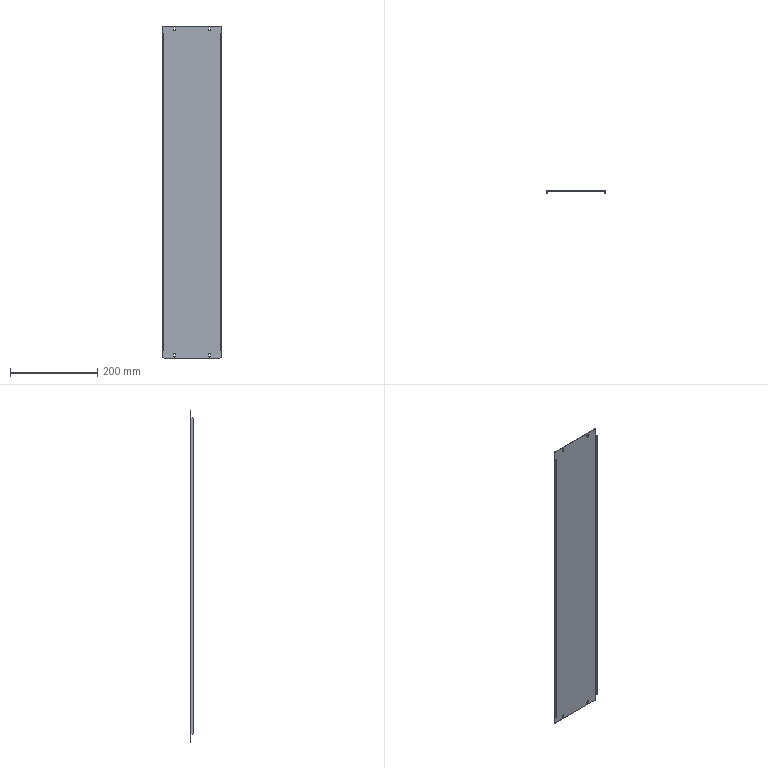Part | SolidWorks | features BaseBody 1 | 1 solid | 42 faces | box 134 x 7.2 x 760 mm | volume 132478 mm3 | plane 22 | cylinder 20 | commonest cylinder face diameters 4 x12 6 x8
STEP:
#1=CARTESIAN_POINT('',(40.,0.,-370.));
#2=VERTEX_POINT('',#1);
#3=CARTESIAN_POINT('',(40.,1.2,-370.));
#4=VERTEX_POINT('',#3);
#5=CARTESIAN_POINT('',(40.,-6.001,-370.));
#6=DIRECTION('',(0.,1.,0.));
#7=VECTOR('',#6,1000.);
#8=LINE('',#5,#7);
#9=EDGE_CURVE('',#2,#4,#8,.T.);
#10=ORIENTED_EDGE('',*,*,#9,.F.);
#11=CARTESIAN_POINT('',(38.,0.,-372.));
#12=VERTEX_POINT('',#11);
#13=CARTESIAN_POINT('',(40.,0.,-372.));
#14=DIRECTION('',(0.,-1.,0.));
#15=DIRECTION('',(0.,0.,1.));
#16=AXIS2_PLACEMENT_3D('',#13,#14,#15);
#17=CIRCLE('',#16,2.);
#18=EDGE_CURVE('',#2,#12,#17,.T.);
#19=ORIENTED_EDGE('',*,*,#18,.T.);
#20=CARTESIAN_POINT('',(38.,1.2,-372.));
#21=VERTEX_POINT('',#20);
#22=CARTESIAN_POINT('',(38.,-6.001,-372.));
#23=DIRECTION('',(0.,1.,0.));
#24=VECTOR('',#23,1000.);
#25=LINE('',#22,#24);
#26=EDGE_CURVE('',#12,#21,#25,.T.);
#27=ORIENTED_EDGE('',*,*,#26,.T.);
#28=CARTESIAN_POINT('',(40.,1.2,-372.));
#29=DIRECTION('',(0.,1.,0.));
#30=DIRECTION('',(0.,0.,1.));
#31=AXIS2_PLACEMENT_3D('',#28,#29,#30);
#32=CIRCLE('',#31,2.);
#33=EDGE_CURVE('',#21,#4,#32,.T.);
#34=ORIENTED_EDGE('',*,*,#33,.T.);
#35=EDGE_LOOP('',(#10,#19,#27,#34));
#36=FACE_OUTER_BOUND('',#35,.T.);
#37=CARTESIAN_POINT('',(40.,-6.001,-372.));
#38=DIRECTION('',(0.,1.,0.));
#39=DIRECTION('',(0.,0.,1.));
#40=AXIS2_PLACEMENT_3D('',#37,#38,#39);
#41=CYLINDRICAL_SURFACE('',#40,2.);
#42=ADVANCED_FACE('',(#36),#41,.F.);
#43=CARTESIAN_POINT('',(-40.,0.,-370.));
#44=VERTEX_POINT('',#43);
#45=CARTESIAN_POINT('',(-40.,1.2,-370.));
#46=VERTEX_POINT('',#45);
#47=CARTESIAN_POINT('',(-40.,-6.001,-370.));
#48=DIRECTION('',(0.,1.,0.));
#49=VECTOR('',#48,1000.);
#50=LINE('',#47,#49);
#51=EDGE_CURVE('',#44,#46,#50,.T.);
#52=ORIENTED_EDGE('',*,*,#51,.F.);
#53=CARTESIAN_POINT('',(-42.,0.,-372.));
#54=VERTEX_POINT('',#53);
#55=CARTESIAN_POINT('',(-40.,0.,-372.));
#56=DIRECTION('',(0.,-1.,0.));
#57=DIRECTION('',(0.,0.,1.));
#58=AXIS2_PLACEMENT_3D('',#55,#56,#57);
#59=CIRCLE('',#58,2.);
#60=EDGE_CURVE('',#44,#54,#59,.T.);
#61=ORIENTED_EDGE('',*,*,#60,.T.);
#62=CARTESIAN_POINT('',(-42.,1.2,-372.));
#63=VERTEX_POINT('',#62);
#64=CARTESIAN_POINT('',(-42.,-6.001,-372.));
#65=DIRECTION('',(0.,1.,0.));
#66=VECTOR('',#65,1000.);
#67=LINE('',#64,#66);
#68=EDGE_CURVE('',#54,#63,#67,.T.);
#69=ORIENTED_EDGE('',*,*,#68,.T.);
#70=CARTESIAN_POINT('',(-40.,1.2,-372.));
#71=DIRECTION('',(0.,1.,0.));
#72=DIRECTION('',(0.,0.,1.));
#73=AXIS2_PLACEMENT_3D('',#70,#71,#72);
#74=CIRCLE('',#73,2.);
#75=EDGE_CURVE('',#63,#46,#74,.T.);
#76=ORIENTED_EDGE('',*,*,#75,.T.);
#77=EDGE_LOOP('',(#52,#61,#69,#76));
#78=FACE_OUTER_BOUND('',#77,.T.);
#79=CARTESIAN_POINT('',(-40.,-6.001,-372.));
#80=DIRECTION('',(0.,1.,0.));
#81=DIRECTION('',(0.,0.,1.));
#82=AXIS2_PLACEMENT_3D('',#79,#80,#81);
#83=CYLINDRICAL_SURFACE('',#82,2.);
#84=ADVANCED_FACE('',(#78),#83,.F.);
#85=CARTESIAN_POINT('',(-42.,0.,372.));
#86=VERTEX_POINT('',#85);
#87=CARTESIAN_POINT('',(-38.,0.,372.));
#88=VERTEX_POINT('',#87);
#89=CARTESIAN_POINT('',(-40.,0.,372.));
#90=DIRECTION('',(0.,-1.,0.));
#91=DIRECTION('',(0.,0.,1.));
#92=AXIS2_PLACEMENT_3D('',#89,#90,#91);
#93=CIRCLE('',#92,2.);
#94=EDGE_CURVE('',#86,#88,#93,.T.);
#95=ORIENTED_EDGE('',*,*,#94,.T.);
#96=CARTESIAN_POINT('',(-38.,1.2,372.));
#97=VERTEX_POINT('',#96);
#98=CARTESIAN_POINT('',(-38.,-6.001,372.));
#99=DIRECTION('',(0.,1.,0.));
#100=VECTOR('',#99,1000.);
#101=LINE('',#98,#100);
#102=EDGE_CURVE('',#88,#97,#101,.T.);
#103=ORIENTED_EDGE('',*,*,#102,.T.);
#104=CARTESIAN_POINT('',(-42.,1.2,372.));
#105=VERTEX_POINT('',#104);
#106=CARTESIAN_POINT('',(-40.,1.2,372.));
#107=DIRECTION('',(0.,1.,0.));
#108=DIRECTION('',(0.,0.,1.));
#109=AXIS2_PLACEMENT_3D('',#106,#107,#108);
#110=CIRCLE('',#109,2.);
#111=EDGE_CURVE('',#97,#105,#110,.T.);
#112=ORIENTED_EDGE('',*,*,#111,.T.);
#113=CARTESIAN_POINT('',(-42.,-6.001,372.));
#114=DIRECTION('',(0.,1.,0.));
#115=VECTOR('',#114,1000.);
#116=LINE('',#113,#115);
#117=EDGE_CURVE('',#86,#105,#116,.T.);
#118=ORIENTED_EDGE('',*,*,#117,.F.);
#119=EDGE_LOOP('',(#95,#103,#112,#118));
#120=FACE_OUTER_BOUND('',#119,.T.);
#121=CARTESIAN_POINT('',(-40.,-6.001,372.));
#122=DIRECTION('',(0.,1.,0.));
#123=DIRECTION('',(0.,0.,1.));
#124=AXIS2_PLACEMENT_3D('',#121,#122,#123);
#125=CYLINDRICAL_SURFACE('',#124,2.);
#126=ADVANCED_FACE('',(#120),#125,.F.);
#127=CARTESIAN_POINT('',(40.,0.,378.));
#128=VERTEX_POINT('',#127);
#129=CARTESIAN_POINT('',(40.,1.2,378.));
#130=VERTEX_POINT('',#129);
#131=CARTESIAN_POINT('',(40.,-6.001,378.));
#132=DIRECTION('',(0.,1.,0.));
#133=VECTOR('',#132,1000.);
#134=LINE('',#131,#133);
#135=EDGE_CURVE('',#128,#130,#134,.T.);
#136=ORIENTED_EDGE('',*,*,#135,.F.);
#137=CARTESIAN_POINT('',(38.,0.,376.));
#138=VERTEX_POINT('',#137);
#139=CARTESIAN_POINT('',(40.,0.,376.));
#140=DIRECTION('',(0.,-1.,0.));
#141=DIRECTION('',(0.,0.,1.));
#142=AXIS2_PLACEMENT_3D('',#139,#140,#141);
#143=CIRCLE('',#142,2.);
#144=EDGE_CURVE('',#128,#138,#143,.T.);
#145=ORIENTED_EDGE('',*,*,#144,.T.);
#146=CARTESIAN_POINT('',(38.,1.2,376.));
#147=VERTEX_POINT('',#146);
#148=CARTESIAN_POINT('',(38.,-6.001,376.));
#149=DIRECTION('',(0.,1.,0.));
#150=VECTOR('',#149,1000.);
#151=LINE('',#148,#150);
#152=EDGE_CURVE('',#138,#147,#151,.T.);
#153=ORIENTED_EDGE('',*,*,#152,.T.);
#154=CARTESIAN_POINT('',(40.,1.2,376.));
#155=DIRECTION('',(0.,1.,0.));
#156=DIRECTION('',(0.,0.,1.));
#157=AXIS2_PLACEMENT_3D('',#154,#155,#156);
#158=CIRCLE('',#157,2.);
#159=EDGE_CURVE('',#147,#130,#158,.T.);
#160=ORIENTED_EDGE('',*,*,#159,.T.);
#161=EDGE_LOOP('',(#136,#145,#153,#160));
#162=FACE_OUTER_BOUND('',#161,.T.);
#163=CARTESIAN_POINT('',(40.,-6.001,376.));
#164=DIRECTION('',(0.,1.,0.));
#165=DIRECTION('',(0.,0.,1.));
#166=AXIS2_PLACEMENT_3D('',#163,#164,#165);
#167=CYLINDRICAL_SURFACE('',#166,2.);
#168=ADVANCED_FACE('',(#162),#167,.F.);
#169=CARTESIAN_POINT('',(38.,0.,372.));
#170=VERTEX_POINT('',#169);
#171=CARTESIAN_POINT('',(38.,0.,372.));
#172=DIRECTION('',(0.,0.,-1.));
#173=VECTOR('',#172,1000.);
#174=LINE('',#171,#173);
#175=EDGE_CURVE('',#138,#170,#174,.T.);
#176=ORIENTED_EDGE('',*,*,#175,.T.);
#177=CARTESIAN_POINT('',(38.,1.2,372.));
#178=VERTEX_POINT('',#177);
#179=CARTESIAN_POINT('',(38.,-6.001,372.));
#180=DIRECTION('',(0.,1.,0.));
#181=VECTOR('',#180,1000.);
#182=LINE('',#179,#181);
#183=EDGE_CURVE('',#170,#178,#182,.T.);
#184=ORIENTED_EDGE('',*,*,#183,.T.);
#185=CARTESIAN_POINT('',(38.,1.2,372.));
#186=DIRECTION('',(0.,0.,1.));
#187=VECTOR('',#186,1000.);
#188=LINE('',#185,#187);
#189=EDGE_CURVE('',#178,#147,#188,.T.);
#190=ORIENTED_EDGE('',*,*,#189,.T.);
#191=ORIENTED_EDGE('',*,*,#152,.F.);
#192=EDGE_LOOP('',(#176,#184,#190,#191));
#193=FACE_OUTER_BOUND('',#192,.T.);
#194=CARTESIAN_POINT('',(38.,-6.001,372.));
#195=DIRECTION('',(-1.,0.,0.));
#196=DIRECTION('',(0.,0.,1.));
#197=AXIS2_PLACEMENT_3D('',#194,#195,#196);
#198=PLANE('',#197);
#199=ADVANCED_FACE('',(#193),#198,.F.);
#200=CARTESIAN_POINT('',(42.,0.,372.));
#201=VERTEX_POINT('',#200);
#202=CARTESIAN_POINT('',(42.,0.,376.));
#203=VERTEX_POINT('',#202);
#204=CARTESIAN_POINT('',(42.,0.,372.));
#205=DIRECTION('',(0.,0.,1.));
#206=VECTOR('',#205,1000.);
#207=LINE('',#204,#206);
#208=EDGE_CURVE('',#201,#203,#207,.T.);
#209=ORIENTED_EDGE('',*,*,#208,.T.);
#210=CARTESIAN_POINT('',(42.,1.2,376.));
#211=VERTEX_POINT('',#210);
#212=CARTESIAN_POINT('',(42.,-6.001,376.));
#213=DIRECTION('',(0.,1.,0.));
#214=VECTOR('',#213,1000.);
#215=LINE('',#212,#214);
#216=EDGE_CURVE('',#203,#211,#215,.T.);
#217=ORIENTED_EDGE('',*,*,#216,.T.);
#218=CARTESIAN_POINT('',(42.,1.2,372.));
#219=VERTEX_POINT('',#218);
#220=CARTESIAN_POINT('',(42.,1.2,372.));
#221=DIRECTION('',(0.,0.,-1.));
#222=VECTOR('',#221,1000.);
#223=LINE('',#220,#222);
#224=EDGE_CURVE('',#211,#219,#223,.T.);
#225=ORIENTED_EDGE('',*,*,#224,.T.);
#226=CARTESIAN_POINT('',(42.,-6.001,372.));
#227=DIRECTION('',(0.,1.,0.));
#228=VECTOR('',#227,1000.);
#229=LINE('',#226,#228);
#230=EDGE_CURVE('',#201,#219,#229,.T.);
#231=ORIENTED_EDGE('',*,*,#230,.F.);
#232=EDGE_LOOP('',(#209,#217,#225,#231));
#233=FACE_OUTER_BOUND('',#232,.T.);
#234=CARTESIAN_POINT('',(42.,-6.001,372.));
#235=DIRECTION('',(1.,0.,0.));
#236=DIRECTION('',(0.,1.,0.));
#237=AXIS2_PLACEMENT_3D('',#234,#235,#236);
#238=PLANE('',#237);
#239=ADVANCED_FACE('',(#233),#238,.F.);
#240=CARTESIAN_POINT('',(40.,0.,372.));
#241=DIRECTION('',(0.,-1.,0.));
#242=DIRECTION('',(0.,0.,1.));
#243=AXIS2_PLACEMENT_3D('',#240,#241,#242);
#244=CIRCLE('',#243,2.);
#245=EDGE_CURVE('',#170,#201,#244,.T.);
#246=ORIENTED_EDGE('',*,*,#245,.T.);
#247=ORIENTED_EDGE('',*,*,#230,.T.);
#248=CARTESIAN_POINT('',(40.,1.2,372.));
#249=DIRECTION('',(0.,1.,0.));
#250=DIRECTION('',(0.,0.,1.));
#251=AXIS2_PLACEMENT_3D('',#248,#249,#250);
#252=CIRCLE('',#251,2.);
#253=EDGE_CURVE('',#219,#178,#252,.T.);
#254=ORIENTED_EDGE('',*,*,#253,.T.);
#255=ORIENTED_EDGE('',*,*,#183,.F.);
#256=EDGE_LOOP('',(#246,#247,#254,#255));
#257=FACE_OUTER_BOUND('',#256,.T.);
#258=CARTESIAN_POINT('',(40.,-6.001,372.));
#259=DIRECTION('',(0.,1.,0.));
#260=DIRECTION('',(0.,0.,1.));
#261=AXIS2_PLACEMENT_3D('',#258,#259,#260);
#262=CYLINDRICAL_SURFACE('',#261,2.);
#263=ADVANCED_FACE('',(#257),#262,.F.);
#264=CARTESIAN_POINT('',(-38.,0.,376.));
#265=VERTEX_POINT('',#264);
#266=CARTESIAN_POINT('',(-38.,0.,372.));
#267=DIRECTION('',(0.,0.,1.));
#268=VECTOR('',#267,1000.);
#269=LINE('',#266,#268);
#270=EDGE_CURVE('',#88,#265,#269,.T.);
#271=ORIENTED_EDGE('',*,*,#270,.T.);
#272=CARTESIAN_POINT('',(-38.,1.2,376.));
#273=VERTEX_POINT('',#272);
#274=CARTESIAN_POINT('',(-38.,-6.001,376.));
#275=DIRECTION('',(0.,1.,0.));
#276=VECTOR('',#275,1000.);
#277=LINE('',#274,#276);
#278=EDGE_CURVE('',#265,#273,#277,.T.);
#279=ORIENTED_EDGE('',*,*,#278,.T.);
#280=CARTESIAN_POINT('',(-38.,1.2,372.));
#281=DIRECTION('',(0.,0.,-1.));
#282=VECTOR('',#281,1000.);
#283=LINE('',#280,#282);
#284=EDGE_CURVE('',#273,#97,#283,.T.);
#285=ORIENTED_EDGE('',*,*,#284,.T.);
#286=ORIENTED_EDGE('',*,*,#102,.F.);
#287=EDGE_LOOP('',(#271,#279,#285,#286));
#288=FACE_OUTER_BOUND('',#287,.T.);
#289=CARTESIAN_POINT('',(-38.,-6.001,372.));
#290=DIRECTION('',(1.,0.,0.));
#291=DIRECTION('',(0.,1.,0.));
#292=AXIS2_PLACEMENT_3D('',#289,#290,#291);
#293=PLANE('',#292);
#294=ADVANCED_FACE('',(#288),#293,.F.);
#295=CARTESIAN_POINT('',(-40.,0.,378.));
#296=VERTEX_POINT('',#295);
#297=CARTESIAN_POINT('',(-40.,1.2,378.));
#298=VERTEX_POINT('',#297);
#299=CARTESIAN_POINT('',(-40.,-6.001,378.));
#300=DIRECTION('',(0.,1.,0.));
#301=VECTOR('',#300,1000.);
#302=LINE('',#299,#301);
#303=EDGE_CURVE('',#296,#298,#302,.T.);
#304=ORIENTED_EDGE('',*,*,#303,.F.);
#305=CARTESIAN_POINT('',(-42.,0.,376.));
#306=VERTEX_POINT('',#305);
#307=CARTESIAN_POINT('',(-40.,0.,376.));
#308=DIRECTION('',(0.,-1.,0.));
#309=DIRECTION('',(0.,0.,1.));
#310=AXIS2_PLACEMENT_3D('',#307,#308,#309);
#311=CIRCLE('',#310,2.);
#312=EDGE_CURVE('',#296,#306,#311,.T.);
#313=ORIENTED_EDGE('',*,*,#312,.T.);
#314=CARTESIAN_POINT('',(-42.,1.2,376.));
#315=VERTEX_POINT('',#314);
#316=CARTESIAN_POINT('',(-42.,-6.001,376.));
#317=DIRECTION('',(0.,1.,0.));
#318=VECTOR('',#317,1000.);
#319=LINE('',#316,#318);
#320=EDGE_CURVE('',#306,#315,#319,.T.);
#321=ORIENTED_EDGE('',*,*,#320,.T.);
#322=CARTESIAN_POINT('',(-40.,1.2,376.));
#323=DIRECTION('',(0.,1.,0.));
#324=DIRECTION('',(0.,0.,1.));
#325=AXIS2_PLACEMENT_3D('',#322,#323,#324);
#326=CIRCLE('',#325,2.);
#327=EDGE_CURVE('',#315,#298,#326,.T.);
#328=ORIENTED_EDGE('',*,*,#327,.T.);
#329=EDGE_LOOP('',(#304,#313,#321,#328));
#330=FACE_OUTER_BOUND('',#329,.T.);
#331=CARTESIAN_POINT('',(-40.,-6.001,376.));
#332=DIRECTION('',(0.,1.,0.));
#333=DIRECTION('',(0.,0.,1.));
#334=AXIS2_PLACEMENT_3D('',#331,#332,#333);
#335=CYLINDRICAL_SURFACE('',#334,2.);
#336=ADVANCED_FACE('',(#330),#335,.F.);
#337=CARTESIAN_POINT('',(-42.,0.,372.));
#338=DIRECTION('',(0.,0.,-1.));
#339=VECTOR('',#338,1000.);
#340=LINE('',#337,#339);
#341=EDGE_CURVE('',#306,#86,#340,.T.);
#342=ORIENTED_EDGE('',*,*,#341,.T.);
#343=ORIENTED_EDGE('',*,*,#117,.T.);
#344=CARTESIAN_POINT('',(-42.,1.2,372.));
#345=DIRECTION('',(0.,0.,1.));
#346=VECTOR('',#345,1000.);
#347=LINE('',#344,#346);
#348=EDGE_CURVE('',#105,#315,#347,.T.);
#349=ORIENTED_EDGE('',*,*,#348,.T.);
#350=ORIENTED_EDGE('',*,*,#320,.F.);
#351=EDGE_LOOP('',(#342,#343,#349,#350));
#352=FACE_OUTER_BOUND('',#351,.T.);
#353=CARTESIAN_POINT('',(-42.,-6.001,372.));
#354=DIRECTION('',(-1.,0.,0.));
#355=DIRECTION('',(0.,0.,1.));
#356=AXIS2_PLACEMENT_3D('',#353,#354,#355);
#357=PLANE('',#356);
#358=ADVANCED_FACE('',(#352),#357,.F.);
#359=CARTESIAN_POINT('',(-42.,0.,-376.));
#360=VERTEX_POINT('',#359);
#361=CARTESIAN_POINT('',(-42.,0.,-376.));
#362=DIRECTION('',(0.,0.,-1.));
#363=VECTOR('',#362,1000.);
#364=LINE('',#361,#363);
#365=EDGE_CURVE('',#54,#360,#364,.T.);
#366=ORIENTED_EDGE('',*,*,#365,.T.);
#367=CARTESIAN_POINT('',(-42.,1.2,-376.));
#368=VERTEX_POINT('',#367);
#369=CARTESIAN_POINT('',(-42.,-6.001,-376.));
#370=DIRECTION('',(0.,1.,0.));
#371=VECTOR('',#370,1000.);
#372=LINE('',#369,#371);
#373=EDGE_CURVE('',#360,#368,#372,.T.);
#374=ORIENTED_EDGE('',*,*,#373,.T.);
#375=CARTESIAN_POINT('',(-42.,1.2,-376.));
#376=DIRECTION('',(0.,0.,1.));
#377=VECTOR('',#376,1000.);
#378=LINE('',#375,#377);
#379=EDGE_CURVE('',#368,#63,#378,.T.);
#380=ORIENTED_EDGE('',*,*,#379,.T.);
#381=ORIENTED_EDGE('',*,*,#68,.F.);
#382=EDGE_LOOP('',(#366,#374,#380,#381));
#383=FACE_OUTER_BOUND('',#382,.T.);
#384=CARTESIAN_POINT('',(-42.,-6.001,-376.));
#385=DIRECTION('',(-1.,0.,0.));
#386=DIRECTION('',(0.,0.,1.));
#387=AXIS2_PLACEMENT_3D('',#384,#385,#386);
#388=PLANE('',#387);
#389=ADVANCED_FACE('',(#383),#388,.F.);
#390=CARTESIAN_POINT('',(-38.,0.,-376.));
#391=VERTEX_POINT('',#390);
#392=CARTESIAN_POINT('',(-38.,0.,-372.));
#393=VERTEX_POINT('',#392);
#394=CARTESIAN_POINT('',(-38.,0.,-376.));
#395=DIRECTION('',(0.,0.,1.));
#396=VECTOR('',#395,1000.);
#397=LINE('',#394,#396);
#398=EDGE_CURVE('',#391,#393,#397,.T.);
#399=ORIENTED_EDGE('',*,*,#398,.T.);
#400=CARTESIAN_POINT('',(-38.,1.2,-372.));
#401=VERTEX_POINT('',#400);
#402=CARTESIAN_POINT('',(-38.,-6.001,-372.));
#403=DIRECTION('',(0.,1.,0.));
#404=VECTOR('',#403,1000.);
#405=LINE('',#402,#404);
#406=EDGE_CURVE('',#393,#401,#405,.T.);
#407=ORIENTED_EDGE('',*,*,#406,.T.);
#408=CARTESIAN_POINT('',(-38.,1.2,-376.));
#409=VERTEX_POINT('',#408);
#410=CARTESIAN_POINT('',(-38.,1.2,-376.));
#411=DIRECTION('',(0.,0.,-1.));
#412=VECTOR('',#411,1000.);
#413=LINE('',#410,#412);
#414=EDGE_CURVE('',#401,#409,#413,.T.);
#415=ORIENTED_EDGE('',*,*,#414,.T.);
#416=CARTESIAN_POINT('',(-38.,-6.001,-376.));
#417=DIRECTION('',(0.,1.,0.));
#418=VECTOR('',#417,1000.);
#419=LINE('',#416,#418);
#420=EDGE_CURVE('',#391,#409,#419,.T.);
#421=ORIENTED_EDGE('',*,*,#420,.F.);
#422=EDGE_LOOP('',(#399,#407,#415,#421));
#423=FACE_OUTER_BOUND('',#422,.T.);
#424=CARTESIAN_POINT('',(-38.,-6.001,-376.));
#425=DIRECTION('',(1.,0.,0.));
#426=DIRECTION('',(0.,1.,0.));
#427=AXIS2_PLACEMENT_3D('',#424,#425,#426);
#428=PLANE('',#427);
#429=ADVANCED_FACE('',(#423),#428,.F.);
#430=CARTESIAN_POINT('',(-40.,0.,-376.));
#431=DIRECTION('',(0.,-1.,0.));
#432=DIRECTION('',(0.,0.,1.));
#433=AXIS2_PLACEMENT_3D('',#430,#431,#432);
#434=CIRCLE('',#433,2.);
#435=EDGE_CURVE('',#360,#391,#434,.T.);
#436=ORIENTED_EDGE('',*,*,#435,.T.);
#437=ORIENTED_EDGE('',*,*,#420,.T.);
#438=CARTESIAN_POINT('',(-40.,1.2,-376.));
#439=DIRECTION('',(0.,1.,0.));
#440=DIRECTION('',(0.,0.,1.));
#441=AXIS2_PLACEMENT_3D('',#438,#439,#440);
#442=CIRCLE('',#441,2.);
#443=EDGE_CURVE('',#409,#368,#442,.T.);
#444=ORIENTED_EDGE('',*,*,#443,.T.);
#445=ORIENTED_EDGE('',*,*,#373,.F.);
#446=EDGE_LOOP('',(#436,#437,#444,#445));
#447=FACE_OUTER_BOUND('',#446,.T.);
#448=CARTESIAN_POINT('',(-40.,-6.001,-376.));
#449=DIRECTION('',(0.,1.,0.));
#450=DIRECTION('',(0.,0.,1.));
#451=AXIS2_PLACEMENT_3D('',#448,#449,#450);
#452=CYLINDRICAL_SURFACE('',#451,2.);
#453=ADVANCED_FACE('',(#447),#452,.F.);
#454=CARTESIAN_POINT('',(38.,0.,-376.));
#455=VERTEX_POINT('',#454);
#456=CARTESIAN_POINT('',(38.,0.,-376.));
#457=DIRECTION('',(0.,0.,-1.));
#458=VECTOR('',#457,1000.);
#459=LINE('',#456,#458);
#460=EDGE_CURVE('',#12,#455,#459,.T.);
#461=ORIENTED_EDGE('',*,*,#460,.T.);
#462=CARTESIAN_POINT('',(38.,1.2,-376.));
#463=VERTEX_POINT('',#462);
#464=CARTESIAN_POINT('',(38.,-6.001,-376.));
#465=DIRECTION('',(0.,1.,0.));
#466=VECTOR('',#465,1000.);
#467=LINE('',#464,#466);
#468=EDGE_CURVE('',#455,#463,#467,.T.);
#469=ORIENTED_EDGE('',*,*,#468,.T.);
#470=CARTESIAN_POINT('',(38.,1.2,-376.));
#471=DIRECTION('',(0.,0.,1.));
#472=VECTOR('',#471,1000.);
#473=LINE('',#470,#472);
#474=EDGE_CURVE('',#463,#21,#473,.T.);
#475=ORIENTED_EDGE('',*,*,#474,.T.);
#476=ORIENTED_EDGE('',*,*,#26,.F.);
#477=EDGE_LOOP('',(#461,#469,#475,#476));
#478=FACE_OUTER_BOUND('',#477,.T.);
#479=CARTESIAN_POINT('',(38.,-6.001,-376.));
#480=DIRECTION('',(-1.,0.,0.));
#481=DIRECTION('',(0.,0.,1.));
#482=AXIS2_PLACEMENT_3D('',#479,#480,#481);
#483=PLANE('',#482);
#484=ADVANCED_FACE('',(#478),#483,.F.);
#485=CARTESIAN_POINT('',(42.,0.,-376.));
#486=VERTEX_POINT('',#485);
#487=CARTESIAN_POINT('',(42.,0.,-372.));
#488=VERTEX_POINT('',#487);
#489=CARTESIAN_POINT('',(42.,0.,-376.));
#490=DIRECTION('',(0.,0.,1.));
#491=VECTOR('',#490,1000.);
#492=LINE('',#489,#491);
#493=EDGE_CURVE('',#486,#488,#492,.T.);
#494=ORIENTED_EDGE('',*,*,#493,.T.);
#495=CARTESIAN_POINT('',(42.,1.2,-372.));
#496=VERTEX_POINT('',#495);
#497=CARTESIAN_POINT('',(42.,-6.001,-372.));
#498=DIRECTION('',(0.,1.,0.));
#499=VECTOR('',#498,1000.);
#500=LINE('',#497,#499);
#501=EDGE_CURVE('',#488,#496,#500,.T.);
#502=ORIENTED_EDGE('',*,*,#501,.T.);
#503=CARTESIAN_POINT('',(42.,1.2,-376.));
#504=VERTEX_POINT('',#503);
#505=CARTESIAN_POINT('',(42.,1.2,-376.));
#506=DIRECTION('',(0.,0.,-1.));
#507=VECTOR('',#506,1000.);
#508=LINE('',#505,#507);
#509=EDGE_CURVE('',#496,#504,#508,.T.);
#510=ORIENTED_EDGE('',*,*,#509,.T.);
#511=CARTESIAN_POINT('',(42.,-6.001,-376.));
#512=DIRECTION('',(0.,1.,0.));
#513=VECTOR('',#512,1000.);
#514=LINE('',#511,#513);
#515=EDGE_CURVE('',#486,#504,#514,.T.);
#516=ORIENTED_EDGE('',*,*,#515,.F.);
#517=EDGE_LOOP('',(#494,#502,#510,#516));
#518=FACE_OUTER_BOUND('',#517,.T.);
#519=CARTESIAN_POINT('',(42.,-6.001,-376.));
#520=DIRECTION('',(1.,0.,0.));
#521=DIRECTION('',(0.,1.,0.));
#522=AXIS2_PLACEMENT_3D('',#519,#520,#521);
#523=PLANE('',#522);
#524=ADVANCED_FACE('',(#518),#523,.F.);
#525=CARTESIAN_POINT('',(40.,0.,-376.));
#526=DIRECTION('',(0.,-1.,0.));
#527=DIRECTION('',(0.,0.,1.));
#528=AXIS2_PLACEMENT_3D('',#525,#526,#527);
#529=CIRCLE('',#528,2.);
#530=EDGE_CURVE('',#455,#486,#529,.T.);
#531=ORIENTED_EDGE('',*,*,#530,.T.);
#532=ORIENTED_EDGE('',*,*,#515,.T.);
#533=CARTESIAN_POINT('',(40.,1.2,-376.));
#534=DIRECTION('',(0.,1.,0.));
#535=DIRECTION('',(0.,0.,1.));
#536=AXIS2_PLACEMENT_3D('',#533,#534,#535);
#537=CIRCLE('',#536,2.);
#538=EDGE_CURVE('',#504,#463,#537,.T.);
#539=ORIENTED_EDGE('',*,*,#538,.T.);
#540=ORIENTED_EDGE('',*,*,#468,.F.);
#541=EDGE_LOOP('',(#531,#532,#539,#540));
#542=FACE_OUTER_BOUND('',#541,.T.);
#543=CARTESIAN_POINT('',(40.,-6.001,-376.));
#544=DIRECTION('',(0.,1.,0.));
#545=DIRECTION('',(0.,0.,1.));
#546=AXIS2_PLACEMENT_3D('',#543,#544,#545);
#547=CYLINDRICAL_SURFACE('',#546,2.);
#548=ADVANCED_FACE('',(#542),#547,.F.);
#549=CARTESIAN_POINT('',(64.,1.2,380.));
#550=VERTEX_POINT('',#549);
#551=CARTESIAN_POINT('',(67.,1.2,377.));
#552=VERTEX_POINT('',#551);
#553=CARTESIAN_POINT('',(64.,1.2,377.));
#554=DIRECTION('',(0.,1.,0.));
#555=DIRECTION('',(0.,0.,1.));
#556=AXIS2_PLACEMENT_3D('',#553,#554,#555);
#557=CIRCLE('',#556,3.);
#558=EDGE_CURVE('',#550,#552,#557,.T.);
#559=ORIENTED_EDGE('',*,*,#558,.F.);
#560=CARTESIAN_POINT('',(64.,0.,380.));
#561=VERTEX_POINT('',#560);
#562=CARTESIAN_POINT('',(64.,1.2,380.));
#563=DIRECTION('',(0.,1.,0.));
#564=VECTOR('',#563,1000.);
#565=LINE('',#562,#564);
#566=EDGE_CURVE('',#561,#550,#565,.T.);
#567=ORIENTED_EDGE('',*,*,#566,.F.);
#568=CARTESIAN_POINT('',(67.,0.,377.));
#569=VERTEX_POINT('',#568);
#570=CARTESIAN_POINT('',(64.,0.,377.));
#571=DIRECTION('',(0.,-1.,0.));
#572=DIRECTION('',(0.,0.,1.));
#573=AXIS2_PLACEMENT_3D('',#570,#571,#572);
#574=CIRCLE('',#573,3.);
#575=EDGE_CURVE('',#569,#561,#574,.T.);
#576=ORIENTED_EDGE('',*,*,#575,.F.);
#577=CARTESIAN_POINT('',(67.,1.2,377.));
#578=DIRECTION('',(0.,-1.,0.));
#579=VECTOR('',#578,1000.);
#580=LINE('',#577,#579);
#581=EDGE_CURVE('',#552,#569,#580,.T.);
#582=ORIENTED_EDGE('',*,*,#581,.F.);
#583=EDGE_LOOP('',(#559,#567,#576,#582));
#584=FACE_OUTER_BOUND('',#583,.T.);
#585=CARTESIAN_POINT('',(64.,1.2,377.));
#586=DIRECTION('',(0.,-1.,0.));
#587=DIRECTION('',(0.,0.,-1.));
#588=AXIS2_PLACEMENT_3D('',#585,#586,#587);
#589=CYLINDRICAL_SURFACE('',#588,3.);
#590=ADVANCED_FACE('',(#584),#589,.T.);
#591=CARTESIAN_POINT('',(65.8,-6.,359.));
#592=VERTEX_POINT('',#591);
#593=CARTESIAN_POINT('',(65.8,-3.,362.));
#594=VERTEX_POINT('',#593);
#595=CARTESIAN_POINT('',(65.8,-3.,359.));
#596=DIRECTION('',(-1.,0.,0.));
#597=DIRECTION('',(0.,0.,-1.));
#598=AXIS2_PLACEMENT_3D('',#595,#596,#597);
#599=CIRCLE('',#598,3.);
#600=EDGE_CURVE('',#592,#594,#599,.T.);
#601=ORIENTED_EDGE('',*,*,#600,.F.);
#602=CARTESIAN_POINT('',(67.,-6.,359.));
#603=VERTEX_POINT('',#602);
#604=CARTESIAN_POINT('',(0.,-6.,359.));
#605=DIRECTION('',(-1.,0.,0.));
#606=VECTOR('',#605,1000.);
#607=LINE('',#604,#606);
#608=EDGE_CURVE('',#603,#592,#607,.T.);
#609=ORIENTED_EDGE('',*,*,#608,.F.);
#610=CARTESIAN_POINT('',(67.,-3.,362.));
#611=VERTEX_POINT('',#610);
#612=CARTESIAN_POINT('',(67.,-3.,359.));
#613=DIRECTION('',(1.,0.,0.));
#614=DIRECTION('',(0.,0.,1.));
#615=AXIS2_PLACEMENT_3D('',#612,#613,#614);
#616=CIRCLE('',#615,3.);
#617=EDGE_CURVE('',#611,#603,#616,.T.);
#618=ORIENTED_EDGE('',*,*,#617,.F.);
#619=CARTESIAN_POINT('',(-67.,-3.,362.));
#620=DIRECTION('',(1.,0.,0.));
#621=VECTOR('',#620,1000.);
#622=LINE('',#619,#621);
#623=EDGE_CURVE('',#594,#611,#622,.T.);
#624=ORIENTED_EDGE('',*,*,#623,.F.);
#625=EDGE_LOOP('',(#601,#609,#618,#624));
#626=FACE_OUTER_BOUND('',#625,.T.);
#627=CARTESIAN_POINT('',(-67.,-3.,359.));
#628=DIRECTION('',(1.,0.,0.));
#629=DIRECTION('',(0.,0.,-1.));
#630=AXIS2_PLACEMENT_3D('',#627,#628,#629);
#631=CYLINDRICAL_SURFACE('',#630,3.);
#632=ADVANCED_FACE('',(#626),#631,.T.);
#633=CARTESIAN_POINT('',(-67.,1.2,377.));
#634=VERTEX_POINT('',#633);
#635=CARTESIAN_POINT('',(-64.,1.2,380.));
#636=VERTEX_POINT('',#635);
#637=CARTESIAN_POINT('',(-64.,1.2,377.));
#638=DIRECTION('',(0.,1.,0.));
#639=DIRECTION('',(0.,0.,1.));
#640=AXIS2_PLACEMENT_3D('',#637,#638,#639);
#641=CIRCLE('',#640,3.);
#642=EDGE_CURVE('',#634,#636,#641,.T.);
#643=ORIENTED_EDGE('',*,*,#642,.F.);
#644=CARTESIAN_POINT('',(-67.,0.,377.));
#645=VERTEX_POINT('',#644);
#646=CARTESIAN_POINT('',(-67.,1.2,377.));
#647=DIRECTION('',(0.,1.,0.));
#648=VECTOR('',#647,1000.);
#649=LINE('',#646,#648);
#650=EDGE_CURVE('',#645,#634,#649,.T.);
#651=ORIENTED_EDGE('',*,*,#650,.F.);
#652=CARTESIAN_POINT('',(-64.,0.,380.));
#653=VERTEX_POINT('',#652);
#654=CARTESIAN_POINT('',(-64.,0.,377.));
#655=DIRECTION('',(0.,-1.,0.));
#656=DIRECTION('',(0.,0.,1.));
#657=AXIS2_PLACEMENT_3D('',#654,#655,#656);
#658=CIRCLE('',#657,3.);
#659=EDGE_CURVE('',#653,#645,#658,.T.);
#660=ORIENTED_EDGE('',*,*,#659,.F.);
#661=CARTESIAN_POINT('',(-64.,1.2,380.));
#662=DIRECTION('',(0.,-1.,0.));
#663=VECTOR('',#662,1000.);
#664=LINE('',#661,#663);
#665=EDGE_CURVE('',#636,#653,#664,.T.);
#666=ORIENTED_EDGE('',*,*,#665,.F.);
#667=EDGE_LOOP('',(#643,#651,#660,#666));
#668=FACE_OUTER_BOUND('',#667,.T.);
#669=CARTESIAN_POINT('',(-64.,1.2,377.));
#670=DIRECTION('',(0.,-1.,0.));
#671=DIRECTION('',(0.,0.,-1.));
#672=AXIS2_PLACEMENT_3D('',#669,#670,#671);
#673=CYLINDRICAL_SURFACE('',#672,3.);
#674=ADVANCED_FACE('',(#668),#673,.T.);
#675=CARTESIAN_POINT('',(-67.,-6.,359.));
#676=VERTEX_POINT('',#675);
#677=CARTESIAN_POINT('',(-67.,-3.,362.));
#678=VERTEX_POINT('',#677);
#679=CARTESIAN_POINT('',(-67.,-3.,359.));
#680=DIRECTION('',(-1.,0.,0.));
#681=DIRECTION('',(0.,0.,-1.));
#682=AXIS2_PLACEMENT_3D('',#679,#680,#681);
#683=CIRCLE('',#682,3.);
#684=EDGE_CURVE('',#676,#678,#683,.T.);
#685=ORIENTED_EDGE('',*,*,#684,.F.);
#686=CARTESIAN_POINT('',(-65.8,-6.,359.));
#687=VERTEX_POINT('',#686);
#688=CARTESIAN_POINT('',(0.,-6.,359.));
#689=DIRECTION('',(-1.,0.,0.));
#690=VECTOR('',#689,1000.);
#691=LINE('',#688,#690);
#692=EDGE_CURVE('',#687,#676,#691,.T.);
#693=ORIENTED_EDGE('',*,*,#692,.F.);
#694=CARTESIAN_POINT('',(-65.8,-3.,362.));
#695=VERTEX_POINT('',#694);
#696=CARTESIAN_POINT('',(-65.8,-3.,359.));
#697=DIRECTION('',(1.,0.,0.));
#698=DIRECTION('',(0.,0.,-1.));
#699=AXIS2_PLACEMENT_3D('',#696,#697,#698);
#700=CIRCLE('',#699,3.);
#701=EDGE_CURVE('',#695,#687,#700,.T.);
#702=ORIENTED_EDGE('',*,*,#701,.F.);
#703=CARTESIAN_POINT('',(-67.,-3.,362.));
#704=DIRECTION('',(1.,0.,0.));
#705=VECTOR('',#704,1000.);
#706=LINE('',#703,#705);
#707=EDGE_CURVE('',#678,#695,#706,.T.);
#708=ORIENTED_EDGE('',*,*,#707,.F.);
#709=EDGE_LOOP('',(#685,#693,#702,#708));
#710=FACE_OUTER_BOUND('',#709,.T.);
#711=CARTESIAN_POINT('',(-67.,-3.,359.));
#712=DIRECTION('',(1.,0.,0.));
#713=DIRECTION('',(0.,0.,-1.));
#714=AXIS2_PLACEMENT_3D('',#711,#712,#713);
#715=CYLINDRICAL_SURFACE('',#714,3.);
#716=ADVANCED_FACE('',(#710),#715,.T.);
#717=CARTESIAN_POINT('',(-64.,1.2,-380.));
#718=VERTEX_POINT('',#717);
#719=CARTESIAN_POINT('',(-67.,1.2,-377.));
#720=VERTEX_POINT('',#719);
#721=CARTESIAN_POINT('',(-64.,1.2,-377.));
#722=DIRECTION('',(0.,1.,0.));
#723=DIRECTION('',(0.,0.,1.));
#724=AXIS2_PLACEMENT_3D('',#721,#722,#723);
#725=CIRCLE('',#724,3.);
#726=EDGE_CURVE('',#718,#720,#725,.T.);
#727=ORIENTED_EDGE('',*,*,#726,.F.);
#728=CARTESIAN_POINT('',(-64.,0.,-380.));
#729=VERTEX_POINT('',#728);
#730=CARTESIAN_POINT('',(-64.,1.2,-380.));
#731=DIRECTION('',(0.,1.,0.));
#732=VECTOR('',#731,1000.);
#733=LINE('',#730,#732);
#734=EDGE_CURVE('',#729,#718,#733,.T.);
#735=ORIENTED_EDGE('',*,*,#734,.F.);
#736=CARTESIAN_POINT('',(-67.,0.,-377.));
#737=VERTEX_POINT('',#736);
#738=CARTESIAN_POINT('',(-64.,0.,-377.));
#739=DIRECTION('',(0.,-1.,0.));
#740=DIRECTION('',(0.,0.,1.));
#741=AXIS2_PLACEMENT_3D('',#738,#739,#740);
#742=CIRCLE('',#741,3.);
#743=EDGE_CURVE('',#737,#729,#742,.T.);
#744=ORIENTED_EDGE('',*,*,#743,.F.);
#745=CARTESIAN_POINT('',(-67.,1.2,-377.));
#746=DIRECTION('',(0.,-1.,0.));
#747=VECTOR('',#746,1000.);
#748=LINE('',#745,#747);
#749=EDGE_CURVE('',#720,#737,#748,.T.);
#750=ORIENTED_EDGE('',*,*,#749,.F.);
#751=EDGE_LOOP('',(#727,#735,#744,#750));
#752=FACE_OUTER_BOUND('',#751,.T.);
#753=CARTESIAN_POINT('',(-64.,1.2,-377.));
#754=DIRECTION('',(0.,-1.,0.));
#755=DIRECTION('',(0.,0.,-1.));
#756=AXIS2_PLACEMENT_3D('',#753,#754,#755);
#757=CYLINDRICAL_SURFACE('',#756,3.);
#758=ADVANCED_FACE('',(#752),#757,.T.);
#759=CARTESIAN_POINT('',(-67.,-3.,-362.));
#760=VERTEX_POINT('',#759);
#761=CARTESIAN_POINT('',(-67.,-6.,-359.));
#762=VERTEX_POINT('',#761);
#763=CARTESIAN_POINT('',(-67.,-3.,-359.));
#764=DIRECTION('',(-1.,0.,0.));
#765=DIRECTION('',(0.,0.,-1.));
#766=AXIS2_PLACEMENT_3D('',#763,#764,#765);
#767=CIRCLE('',#766,3.);
#768=EDGE_CURVE('',#760,#762,#767,.T.);
#769=ORIENTED_EDGE('',*,*,#768,.F.);
#770=CARTESIAN_POINT('',(-65.8,-3.,-362.));
#771=VERTEX_POINT('',#770);
#772=CARTESIAN_POINT('',(-67.,-3.,-362.));
#773=DIRECTION('',(-1.,0.,0.));
#774=VECTOR('',#773,1000.);
#775=LINE('',#772,#774);
#776=EDGE_CURVE('',#771,#760,#775,.T.);
#777=ORIENTED_EDGE('',*,*,#776,.F.);
#778=CARTESIAN_POINT('',(-65.8,-6.,-359.));
#779=VERTEX_POINT('',#778);
#780=CARTESIAN_POINT('',(-65.8,-3.,-359.));
#781=DIRECTION('',(1.,0.,0.));
#782=DIRECTION('',(0.,0.,-1.));
#783=AXIS2_PLACEMENT_3D('',#780,#781,#782);
#784=CIRCLE('',#783,3.);
#785=EDGE_CURVE('',#779,#771,#784,.T.);
#786=ORIENTED_EDGE('',*,*,#785,.F.);
#787=CARTESIAN_POINT('',(0.,-6.,-359.));
#788=DIRECTION('',(1.,0.,0.));
#789=VECTOR('',#788,1000.);
#790=LINE('',#787,#789);
#791=EDGE_CURVE('',#762,#779,#790,.T.);
#792=ORIENTED_EDGE('',*,*,#791,.F.);
#793=EDGE_LOOP('',(#769,#777,#786,#792));
#794=FACE_OUTER_BOUND('',#793,.T.);
#795=CARTESIAN_POINT('',(0.,-3.,-359.));
#796=DIRECTION('',(1.,0.,0.));
#797=DIRECTION('',(0.,0.,-1.));
#798=AXIS2_PLACEMENT_3D('',#795,#796,#797);
#799=CYLINDRICAL_SURFACE('',#798,3.);
#800=ADVANCED_FACE('',(#794),#799,.T.);
#801=CARTESIAN_POINT('',(67.,1.2,-377.));
#802=VERTEX_POINT('',#801);
#803=CARTESIAN_POINT('',(64.,1.2,-380.));
#804=VERTEX_POINT('',#803);
#805=CARTESIAN_POINT('',(64.,1.2,-377.));
#806=DIRECTION('',(0.,1.,0.));
#807=DIRECTION('',(0.,0.,1.));
#808=AXIS2_PLACEMENT_3D('',#805,#806,#807);
#809=CIRCLE('',#808,3.);
#810=EDGE_CURVE('',#802,#804,#809,.T.);
#811=ORIENTED_EDGE('',*,*,#810,.F.);
#812=CARTESIAN_POINT('',(67.,0.,-377.));
#813=VERTEX_POINT('',#812);
#814=CARTESIAN_POINT('',(67.,1.2,-377.));
#815=DIRECTION('',(0.,1.,0.));
#816=VECTOR('',#815,1000.);
#817=LINE('',#814,#816);
#818=EDGE_CURVE('',#813,#802,#817,.T.);
#819=ORIENTED_EDGE('',*,*,#818,.F.);
#820=CARTESIAN_POINT('',(64.,0.,-380.));
#821=VERTEX_POINT('',#820);
#822=CARTESIAN_POINT('',(64.,0.,-377.));
#823=DIRECTION('',(0.,-1.,0.));
#824=DIRECTION('',(0.,0.,1.));
#825=AXIS2_PLACEMENT_3D('',#822,#823,#824);
#826=CIRCLE('',#825,3.);
#827=EDGE_CURVE('',#821,#813,#826,.T.);
#828=ORIENTED_EDGE('',*,*,#827,.F.);
#829=CARTESIAN_POINT('',(64.,1.2,-380.));
#830=DIRECTION('',(0.,-1.,0.));
#831=VECTOR('',#830,1000.);
#832=LINE('',#829,#831);
#833=EDGE_CURVE('',#804,#821,#832,.T.);
#834=ORIENTED_EDGE('',*,*,#833,.F.);
#835=EDGE_LOOP('',(#811,#819,#828,#834));
#836=FACE_OUTER_BOUND('',#835,.T.);
#837=CARTESIAN_POINT('',(64.,1.2,-377.));
#838=DIRECTION('',(0.,-1.,0.));
#839=DIRECTION('',(0.,0.,-1.));
#840=AXIS2_PLACEMENT_3D('',#837,#838,#839);
#841=CYLINDRICAL_SURFACE('',#840,3.);
#842=ADVANCED_FACE('',(#836),#841,.T.);
#843=CARTESIAN_POINT('',(65.8,-3.,-362.));
#844=VERTEX_POINT('',#843);
#845=CARTESIAN_POINT('',(65.8,-6.,-359.));
#846=VERTEX_POINT('',#845);
#847=CARTESIAN_POINT('',(65.8,-3.,-359.));
#848=DIRECTION('',(-1.,0.,0.));
#849=DIRECTION('',(0.,0.,-1.));
#850=AXIS2_PLACEMENT_3D('',#847,#848,#849);
#851=CIRCLE('',#850,3.);
#852=EDGE_CURVE('',#844,#846,#851,.T.);
#853=ORIENTED_EDGE('',*,*,#852,.F.);
#854=CARTESIAN_POINT('',(67.,-3.,-362.));
#855=VERTEX_POINT('',#854);
#856=CARTESIAN_POINT('',(-67.,-3.,-362.));
#857=DIRECTION('',(-1.,0.,0.));
#858=VECTOR('',#857,1000.);
#859=LINE('',#856,#858);
#860=EDGE_CURVE('',#855,#844,#859,.T.);
#861=ORIENTED_EDGE('',*,*,#860,.F.);
#862=CARTESIAN_POINT('',(67.,-6.,-359.));
#863=VERTEX_POINT('',#862);
#864=CARTESIAN_POINT('',(67.,-3.,-359.));
#865=DIRECTION('',(1.,0.,0.));
#866=DIRECTION('',(0.,0.,1.));
#867=AXIS2_PLACEMENT_3D('',#864,#865,#866);
#868=CIRCLE('',#867,3.);
#869=EDGE_CURVE('',#863,#855,#868,.T.);
#870=ORIENTED_EDGE('',*,*,#869,.F.);
#871=CARTESIAN_POINT('',(0.,-6.,-359.));
#872=DIRECTION('',(1.,0.,0.));
#873=VECTOR('',#872,1000.);
#874=LINE('',#871,#873);
#875=EDGE_CURVE('',#846,#863,#874,.T.);
#876=ORIENTED_EDGE('',*,*,#875,.F.);
#877=EDGE_LOOP('',(#853,#861,#870,#876));
#878=FACE_OUTER_BOUND('',#877,.T.);
#879=CARTESIAN_POINT('',(0.,-3.,-359.));
#880=DIRECTION('',(1.,0.,0.));
#881=DIRECTION('',(0.,0.,-1.));
#882=AXIS2_PLACEMENT_3D('',#879,#880,#881);
#883=CYLINDRICAL_SURFACE('',#882,3.);
#884=ADVANCED_FACE('',(#878),#883,.T.);
#885=CARTESIAN_POINT('',(65.8,0.,362.));
#886=VERTEX_POINT('',#885);
#887=CARTESIAN_POINT('',(65.8,-6.,362.));
#888=DIRECTION('',(0.,1.,0.));
#889=VECTOR('',#888,1000.);
#890=LINE('',#887,#889);
#891=EDGE_CURVE('',#594,#886,#890,.T.);
#892=ORIENTED_EDGE('',*,*,#891,.F.);
#893=ORIENTED_EDGE('',*,*,#623,.T.);
#894=CARTESIAN_POINT('',(67.,0.,362.));
#895=VERTEX_POINT('',#894);
#896=CARTESIAN_POINT('',(67.,0.,362.));
#897=DIRECTION('',(0.,1.,0.));
#898=VECTOR('',#897,1000.);
#899=LINE('',#896,#898);
#900=EDGE_CURVE('',#611,#895,#899,.T.);
#901=ORIENTED_EDGE('',*,*,#900,.T.);
#902=CARTESIAN_POINT('',(-67.,0.,362.));
#903=DIRECTION('',(1.,0.,0.));
#904=VECTOR('',#903,1000.);
#905=LINE('',#902,#904);
#906=EDGE_CURVE('',#886,#895,#905,.T.);
#907=ORIENTED_EDGE('',*,*,#906,.F.);
#908=EDGE_LOOP('',(#892,#893,#901,#907));
#909=FACE_OUTER_BOUND('',#908,.T.);
#910=CARTESIAN_POINT('',(-67.,0.,362.));
#911=DIRECTION('',(0.,0.,-1.));
#912=DIRECTION('',(0.,-1.,0.));
#913=AXIS2_PLACEMENT_3D('',#910,#911,#912);
#914=PLANE('',#913);
#915=ADVANCED_FACE('',(#909),#914,.F.);
#916=CARTESIAN_POINT('',(-67.,0.,362.));
#917=VERTEX_POINT('',#916);
#918=CARTESIAN_POINT('',(-67.,0.,362.));
#919=DIRECTION('',(0.,1.,0.));
#920=VECTOR('',#919,1000.);
#921=LINE('',#918,#920);
#922=EDGE_CURVE('',#678,#917,#921,.T.);
#923=ORIENTED_EDGE('',*,*,#922,.F.);
#924=ORIENTED_EDGE('',*,*,#707,.T.);
#925=CARTESIAN_POINT('',(-65.8,0.,362.));
#926=VERTEX_POINT('',#925);
#927=CARTESIAN_POINT('',(-65.8,-6.,362.));
#928=DIRECTION('',(0.,1.,0.));
#929=VECTOR('',#928,1000.);
#930=LINE('',#927,#929);
#931=EDGE_CURVE('',#695,#926,#930,.T.);
#932=ORIENTED_EDGE('',*,*,#931,.T.);
#933=CARTESIAN_POINT('',(-67.,0.,362.));
#934=DIRECTION('',(1.,0.,0.));
#935=VECTOR('',#934,1000.);
#936=LINE('',#933,#935);
#937=EDGE_CURVE('',#917,#926,#936,.T.);
#938=ORIENTED_EDGE('',*,*,#937,.F.);
#939=EDGE_LOOP('',(#923,#924,#932,#938));
#940=FACE_OUTER_BOUND('',#939,.T.);
#941=CARTESIAN_POINT('',(-67.,0.,362.));
#942=DIRECTION('',(0.,0.,-1.));
#943=DIRECTION('',(0.,-1.,0.));
#944=AXIS2_PLACEMENT_3D('',#941,#942,#943);
#945=PLANE('',#944);
#946=ADVANCED_FACE('',(#940),#945,.F.);
#947=CARTESIAN_POINT('',(67.,0.,-362.));
#948=VERTEX_POINT('',#947);
#949=CARTESIAN_POINT('',(67.,0.,-362.));
#950=DIRECTION('',(0.,-1.,0.));
#951=VECTOR('',#950,1000.);
#952=LINE('',#949,#951);
#953=EDGE_CURVE('',#948,#855,#952,.T.);
#954=ORIENTED_EDGE('',*,*,#953,.T.);
#955=ORIENTED_EDGE('',*,*,#860,.T.);
#956=CARTESIAN_POINT('',(65.8,0.,-362.));
#957=VERTEX_POINT('',#956);
#958=CARTESIAN_POINT('',(65.8,-6.,-362.));
#959=DIRECTION('',(0.,-1.,0.));
#960=VECTOR('',#959,1000.);
#961=LINE('',#958,#960);
#962=EDGE_CURVE('',#957,#844,#961,.T.);
#963=ORIENTED_EDGE('',*,*,#962,.F.);
#964=CARTESIAN_POINT('',(-67.,0.,-362.));
#965=DIRECTION('',(1.,0.,0.));
#966=VECTOR('',#965,1000.);
#967=LINE('',#964,#966);
#968=EDGE_CURVE('',#957,#948,#967,.T.);
#969=ORIENTED_EDGE('',*,*,#968,.T.);
#970=EDGE_LOOP('',(#954,#955,#963,#969));
#971=FACE_OUTER_BOUND('',#970,.T.);
#972=CARTESIAN_POINT('',(-67.,0.,-362.));
#973=DIRECTION('',(0.,0.,1.));
#974=DIRECTION('',(0.,-1.,0.));
#975=AXIS2_PLACEMENT_3D('',#972,#973,#974);
#976=PLANE('',#975);
#977=ADVANCED_FACE('',(#971),#976,.F.);
#978=CARTESIAN_POINT('',(-65.8,0.,-362.));
#979=VERTEX_POINT('',#978);
#980=CARTESIAN_POINT('',(-65.8,-6.,-362.));
#981=DIRECTION('',(0.,-1.,0.));
#982=VECTOR('',#981,1000.);
#983=LINE('',#980,#982);
#984=EDGE_CURVE('',#979,#771,#983,.T.);
#985=ORIENTED_EDGE('',*,*,#984,.T.);
#986=ORIENTED_EDGE('',*,*,#776,.T.);
#987=CARTESIAN_POINT('',(-67.,0.,-362.));
#988=VERTEX_POINT('',#987);
#989=CARTESIAN_POINT('',(-67.,0.,-362.));
#990=DIRECTION('',(0.,-1.,0.));
#991=VECTOR('',#990,1000.);
#992=LINE('',#989,#991);
#993=EDGE_CURVE('',#988,#760,#992,.T.);
#994=ORIENTED_EDGE('',*,*,#993,.F.);
#995=CARTESIAN_POINT('',(-67.,0.,-362.));
#996=DIRECTION('',(1.,0.,0.));
#997=VECTOR('',#996,1000.);
#998=LINE('',#995,#997);
#999=EDGE_CURVE('',#988,#979,#998,.T.);
#1000=ORIENTED_EDGE('',*,*,#999,.T.);
#1001=EDGE_LOOP('',(#985,#986,#994,#1000));
#1002=FACE_OUTER_BOUND('',#1001,.T.);
#1003=CARTESIAN_POINT('',(-67.,0.,-362.));
#1004=DIRECTION('',(0.,0.,1.));
#1005=DIRECTION('',(0.,-1.,0.));
#1006=AXIS2_PLACEMENT_3D('',#1003,#1004,#1005);
#1007=PLANE('',#1006);
#1008=ADVANCED_FACE('',(#1002),#1007,.F.);
#1009=CARTESIAN_POINT('',(-67.,-6.,380.));
#1010=DIRECTION('',(0.,0.,-1.));
#1011=VECTOR('',#1010,1000.);
#1012=LINE('',#1009,#1011);
#1013=EDGE_CURVE('',#676,#762,#1012,.T.);
#1014=ORIENTED_EDGE('',*,*,#1013,.T.);
#1015=ORIENTED_EDGE('',*,*,#791,.T.);
#1016=CARTESIAN_POINT('',(-65.8,-6.,380.));
#1017=DIRECTION('',(0.,0.,-1.));
#1018=VECTOR('',#1017,1000.);
#1019=LINE('',#1016,#1018);
#1020=EDGE_CURVE('',#687,#779,#1019,.T.);
#1021=ORIENTED_EDGE('',*,*,#1020,.F.);
#1022=ORIENTED_EDGE('',*,*,#692,.T.);
#1023=EDGE_LOOP('',(#1014,#1015,#1021,#1022));
#1024=FACE_OUTER_BOUND('',#1023,.T.);
#1025=CARTESIAN_POINT('',(0.,-6.,0.));
#1026=DIRECTION('',(0.,1.,0.));
#1027=DIRECTION('',(1.,0.,0.));
#1028=AXIS2_PLACEMENT_3D('',#1025,#1026,#1027);
#1029=PLANE('',#1028);
#1030=ADVANCED_FACE('',(#1024),#1029,.F.);
#1031=ORIENTED_EDGE('',*,*,#1020,.T.);
#1032=ORIENTED_EDGE('',*,*,#785,.T.);
#1033=ORIENTED_EDGE('',*,*,#984,.F.);
#1034=CARTESIAN_POINT('',(-65.8,0.,380.));
#1035=DIRECTION('',(0.,0.,-1.));
#1036=VECTOR('',#1035,1000.);
#1037=LINE('',#1034,#1036);
#1038=EDGE_CURVE('',#926,#979,#1037,.T.);
#1039=ORIENTED_EDGE('',*,*,#1038,.F.);
#1040=ORIENTED_EDGE('',*,*,#931,.F.);
#1041=ORIENTED_EDGE('',*,*,#701,.T.);
#1042=EDGE_LOOP('',(#1031,#1032,#1033,#1039,#1040,#1041));
#1043=FACE_OUTER_BOUND('',#1042,.T.);
#1044=CARTESIAN_POINT('',(-65.8,-6.,380.));
#1045=DIRECTION('',(1.,0.,0.));
#1046=DIRECTION('',(0.,0.,1.));
#1047=AXIS2_PLACEMENT_3D('',#1044,#1045,#1046);
#1048=PLANE('',#1047);
#1049=ADVANCED_FACE('',(#1043),#1048,.T.);
#1050=CARTESIAN_POINT('',(65.8,-6.,380.));
#1051=DIRECTION('',(0.,0.,-1.));
#1052=VECTOR('',#1051,1000.);
#1053=LINE('',#1050,#1052);
#1054=EDGE_CURVE('',#592,#846,#1053,.T.);
#1055=ORIENTED_EDGE('',*,*,#1054,.T.);
#1056=ORIENTED_EDGE('',*,*,#875,.T.);
#1057=CARTESIAN_POINT('',(67.,-6.,380.));
#1058=DIRECTION('',(0.,0.,-1.));
#1059=VECTOR('',#1058,1000.);
#1060=LINE('',#1057,#1059);
#1061=EDGE_CURVE('',#603,#863,#1060,.T.);
#1062=ORIENTED_EDGE('',*,*,#1061,.F.);
#1063=ORIENTED_EDGE('',*,*,#608,.T.);
#1064=EDGE_LOOP('',(#1055,#1056,#1062,#1063));
#1065=FACE_OUTER_BOUND('',#1064,.T.);
#1066=CARTESIAN_POINT('',(0.,-6.,0.));
#1067=DIRECTION('',(0.,1.,0.));
#1068=DIRECTION('',(1.,0.,0.));
#1069=AXIS2_PLACEMENT_3D('',#1066,#1067,#1068);
#1070=PLANE('',#1069);
#1071=ADVANCED_FACE('',(#1065),#1070,.F.);
#1072=ORIENTED_EDGE('',*,*,#962,.T.);
#1073=ORIENTED_EDGE('',*,*,#852,.T.);
#1074=ORIENTED_EDGE('',*,*,#1054,.F.);
#1075=ORIENTED_EDGE('',*,*,#600,.T.);
#1076=ORIENTED_EDGE('',*,*,#891,.T.);
#1077=CARTESIAN_POINT('',(65.8,0.,380.));
#1078=DIRECTION('',(0.,0.,-1.));
#1079=VECTOR('',#1078,1000.);
#1080=LINE('',#1077,#1079);
#1081=EDGE_CURVE('',#886,#957,#1080,.T.);
#1082=ORIENTED_EDGE('',*,*,#1081,.T.);
#1083=EDGE_LOOP('',(#1072,#1073,#1074,#1075,#1076,#1082));
#1084=FACE_OUTER_BOUND('',#1083,.T.);
#1085=CARTESIAN_POINT('',(65.8,-6.,380.));
#1086=DIRECTION('',(1.,0.,0.));
#1087=DIRECTION('',(0.,0.,-1.));
#1088=AXIS2_PLACEMENT_3D('',#1085,#1086,#1087);
#1089=PLANE('',#1088);
#1090=ADVANCED_FACE('',(#1084),#1089,.F.);
#1091=ORIENTED_EDGE('',*,*,#159,.F.);
#1092=ORIENTED_EDGE('',*,*,#189,.F.);
#1093=ORIENTED_EDGE('',*,*,#253,.F.);
#1094=ORIENTED_EDGE('',*,*,#224,.F.);
#1095=CARTESIAN_POINT('',(40.,1.2,376.));
#1096=DIRECTION('',(0.,1.,0.));
#1097=DIRECTION('',(0.,0.,1.));
#1098=AXIS2_PLACEMENT_3D('',#1095,#1096,#1097);
#1099=CIRCLE('',#1098,2.);
#1100=EDGE_CURVE('',#130,#211,#1099,.T.);
#1101=ORIENTED_EDGE('',*,*,#1100,.F.);
#1102=EDGE_LOOP('',(#1091,#1092,#1093,#1094,#1101));
#1103=FACE_BOUND('',#1102,.T.);
#1104=ORIENTED_EDGE('',*,*,#75,.F.);
#1105=ORIENTED_EDGE('',*,*,#379,.F.);
#1106=ORIENTED_EDGE('',*,*,#443,.F.);
#1107=ORIENTED_EDGE('',*,*,#414,.F.);
#1108=CARTESIAN_POINT('',(-40.,1.2,-372.));
#1109=DIRECTION('',(0.,1.,0.));
#1110=DIRECTION('',(0.,0.,1.));
#1111=AXIS2_PLACEMENT_3D('',#1108,#1109,#1110);
#1112=CIRCLE('',#1111,2.);
#1113=EDGE_CURVE('',#46,#401,#1112,.T.);
#1114=ORIENTED_EDGE('',*,*,#1113,.F.);
#1115=EDGE_LOOP('',(#1104,#1105,#1106,#1107,#1114));
#1116=FACE_BOUND('',#1115,.T.);
#1117=ORIENTED_EDGE('',*,*,#33,.F.);
#1118=ORIENTED_EDGE('',*,*,#474,.F.);
#1119=ORIENTED_EDGE('',*,*,#538,.F.);
#1120=ORIENTED_EDGE('',*,*,#509,.F.);
#1121=CARTESIAN_POINT('',(40.,1.2,-372.));
#1122=DIRECTION('',(0.,1.,0.));
#1123=DIRECTION('',(0.,0.,1.));
#1124=AXIS2_PLACEMENT_3D('',#1121,#1122,#1123);
#1125=CIRCLE('',#1124,2.);
#1126=EDGE_CURVE('',#4,#496,#1125,.T.);
#1127=ORIENTED_EDGE('',*,*,#1126,.F.);
#1128=EDGE_LOOP('',(#1117,#1118,#1119,#1120,#1127));
#1129=FACE_BOUND('',#1128,.T.);
#1130=ORIENTED_EDGE('',*,*,#111,.F.);
#1131=ORIENTED_EDGE('',*,*,#284,.F.);
#1132=CARTESIAN_POINT('',(-40.,1.2,376.));
#1133=DIRECTION('',(0.,1.,0.));
#1134=DIRECTION('',(0.,0.,1.));
#1135=AXIS2_PLACEMENT_3D('',#1132,#1133,#1134);
#1136=CIRCLE('',#1135,2.);
#1137=EDGE_CURVE('',#298,#273,#1136,.T.);
#1138=ORIENTED_EDGE('',*,*,#1137,.F.);
#1139=ORIENTED_EDGE('',*,*,#327,.F.);
#1140=ORIENTED_EDGE('',*,*,#348,.F.);
#1141=EDGE_LOOP('',(#1130,#1131,#1138,#1139,#1140));
#1142=FACE_BOUND('',#1141,.T.);
#1143=CARTESIAN_POINT('',(67.,1.2,-380.));
#1144=DIRECTION('',(0.,0.,-1.));
#1145=VECTOR('',#1144,1000.);
#1146=LINE('',#1143,#1145);
#1147=EDGE_CURVE('',#552,#802,#1146,.T.);
#1148=ORIENTED_EDGE('',*,*,#1147,.T.);
#1149=ORIENTED_EDGE('',*,*,#810,.T.);
#1150=CARTESIAN_POINT('',(-67.,1.2,-380.));
#1151=DIRECTION('',(-1.,0.,0.));
#1152=VECTOR('',#1151,1000.);
#1153=LINE('',#1150,#1152);
#1154=EDGE_CURVE('',#804,#718,#1153,.T.);
#1155=ORIENTED_EDGE('',*,*,#1154,.T.);
#1156=ORIENTED_EDGE('',*,*,#726,.T.);
#1157=CARTESIAN_POINT('',(-67.,1.2,-380.));
#1158=DIRECTION('',(0.,0.,1.));
#1159=VECTOR('',#1158,1000.);
#1160=LINE('',#1157,#1159);
#1161=EDGE_CURVE('',#720,#634,#1160,.T.);
#1162=ORIENTED_EDGE('',*,*,#1161,.T.);
#1163=ORIENTED_EDGE('',*,*,#642,.T.);
#1164=CARTESIAN_POINT('',(-67.,1.2,380.));
#1165=DIRECTION('',(1.,0.,0.));
#1166=VECTOR('',#1165,1000.);
#1167=LINE('',#1164,#1166);
#1168=EDGE_CURVE('',#636,#550,#1167,.T.);
#1169=ORIENTED_EDGE('',*,*,#1168,.T.);
#1170=ORIENTED_EDGE('',*,*,#558,.T.);
#1171=EDGE_LOOP('',(#1148,#1149,#1155,#1156,#1162,#1163,#1169,#1170));
#1172=FACE_OUTER_BOUND('',#1171,.T.);
#1173=CARTESIAN_POINT('',(0.,1.2,0.));
#1174=DIRECTION('',(0.,1.,0.));
#1175=DIRECTION('',(1.,0.,0.));
#1176=AXIS2_PLACEMENT_3D('',#1173,#1174,#1175);
#1177=PLANE('',#1176);
#1178=ADVANCED_FACE('',(#1103,#1116,#1129,#1142,#1172),#1177,.T.);
#1179=ORIENTED_EDGE('',*,*,#1168,.F.);
#1180=ORIENTED_EDGE('',*,*,#665,.T.);
#1181=CARTESIAN_POINT('',(-67.,0.,380.));
#1182=DIRECTION('',(1.,0.,0.));
#1183=VECTOR('',#1182,1000.);
#1184=LINE('',#1181,#1183);
#1185=EDGE_CURVE('',#653,#561,#1184,.T.);
#1186=ORIENTED_EDGE('',*,*,#1185,.T.);
#1187=ORIENTED_EDGE('',*,*,#566,.T.);
#1188=EDGE_LOOP('',(#1179,#1180,#1186,#1187));
#1189=FACE_OUTER_BOUND('',#1188,.T.);
#1190=CARTESIAN_POINT('',(-67.,1.2,380.));
#1191=DIRECTION('',(0.,0.,-1.));
#1192=DIRECTION('',(0.,-1.,0.));
#1193=AXIS2_PLACEMENT_3D('',#1190,#1191,#1192);
#1194=PLANE('',#1193);
#1195=ADVANCED_FACE('',(#1189),#1194,.F.);
#1196=ORIENTED_EDGE('',*,*,#993,.T.);
#1197=ORIENTED_EDGE('',*,*,#768,.T.);
#1198=ORIENTED_EDGE('',*,*,#1013,.F.);
#1199=ORIENTED_EDGE('',*,*,#684,.T.);
#1200=ORIENTED_EDGE('',*,*,#922,.T.);
#1201=CARTESIAN_POINT('',(-67.,0.,380.));
#1202=DIRECTION('',(0.,0.,1.));
#1203=VECTOR('',#1202,1000.);
#1204=LINE('',#1201,#1203);
#1205=EDGE_CURVE('',#917,#645,#1204,.T.);
#1206=ORIENTED_EDGE('',*,*,#1205,.T.);
#1207=ORIENTED_EDGE('',*,*,#650,.T.);
#1208=ORIENTED_EDGE('',*,*,#1161,.F.);
#1209=ORIENTED_EDGE('',*,*,#749,.T.);
#1210=CARTESIAN_POINT('',(-67.,0.,-380.));
#1211=DIRECTION('',(0.,0.,1.));
#1212=VECTOR('',#1211,1000.);
#1213=LINE('',#1210,#1212);
#1214=EDGE_CURVE('',#737,#988,#1213,.T.);
#1215=ORIENTED_EDGE('',*,*,#1214,.T.);
#1216=EDGE_LOOP('',(#1196,#1197,#1198,#1199,#1200,#1206,#1207,#1208,#1209,#1215));
#1217=FACE_OUTER_BOUND('',#1216,.T.);
#1218=CARTESIAN_POINT('',(-67.,1.2,-380.));
#1219=DIRECTION('',(1.,0.,0.));
#1220=DIRECTION('',(0.,0.,-1.));
#1221=AXIS2_PLACEMENT_3D('',#1218,#1219,#1220);
#1222=PLANE('',#1221);
#1223=ADVANCED_FACE('',(#1217),#1222,.F.);
#1224=ORIENTED_EDGE('',*,*,#1154,.F.);
#1225=ORIENTED_EDGE('',*,*,#833,.T.);
#1226=CARTESIAN_POINT('',(-67.,0.,-380.));
#1227=DIRECTION('',(-1.,0.,0.));
#1228=VECTOR('',#1227,1000.);
#1229=LINE('',#1226,#1228);
#1230=EDGE_CURVE('',#821,#729,#1229,.T.);
#1231=ORIENTED_EDGE('',*,*,#1230,.T.);
#1232=ORIENTED_EDGE('',*,*,#734,.T.);
#1233=EDGE_LOOP('',(#1224,#1225,#1231,#1232));
#1234=FACE_OUTER_BOUND('',#1233,.T.);
#1235=CARTESIAN_POINT('',(-67.,1.2,-380.));
#1236=DIRECTION('',(0.,0.,1.));
#1237=DIRECTION('',(1.,0.,0.));
#1238=AXIS2_PLACEMENT_3D('',#1235,#1236,#1237);
#1239=PLANE('',#1238);
#1240=ADVANCED_FACE('',(#1234),#1239,.F.);
#1241=ORIENTED_EDGE('',*,*,#1061,.T.);
#1242=ORIENTED_EDGE('',*,*,#869,.T.);
#1243=ORIENTED_EDGE('',*,*,#953,.F.);
#1244=CARTESIAN_POINT('',(67.,0.,-380.));
#1245=DIRECTION('',(0.,0.,1.));
#1246=VECTOR('',#1245,1000.);
#1247=LINE('',#1244,#1246);
#1248=EDGE_CURVE('',#813,#948,#1247,.T.);
#1249=ORIENTED_EDGE('',*,*,#1248,.F.);
#1250=ORIENTED_EDGE('',*,*,#818,.T.);
#1251=ORIENTED_EDGE('',*,*,#1147,.F.);
#1252=ORIENTED_EDGE('',*,*,#581,.T.);
#1253=CARTESIAN_POINT('',(67.,0.,380.));
#1254=DIRECTION('',(0.,0.,1.));
#1255=VECTOR('',#1254,1000.);
#1256=LINE('',#1253,#1255);
#1257=EDGE_CURVE('',#895,#569,#1256,.T.);
#1258=ORIENTED_EDGE('',*,*,#1257,.F.);
#1259=ORIENTED_EDGE('',*,*,#900,.F.);
#1260=ORIENTED_EDGE('',*,*,#617,.T.);
#1261=EDGE_LOOP('',(#1241,#1242,#1243,#1249,#1250,#1251,#1252,#1258,#1259,#1260));
#1262=FACE_OUTER_BOUND('',#1261,.T.);
#1263=CARTESIAN_POINT('',(67.,1.2,-380.));
#1264=DIRECTION('',(-1.,0.,0.));
#1265=DIRECTION('',(0.,1.,0.));
#1266=AXIS2_PLACEMENT_3D('',#1263,#1264,#1265);
#1267=PLANE('',#1266);
#1268=ADVANCED_FACE('',(#1262),#1267,.F.);
#1269=ORIENTED_EDGE('',*,*,#175,.F.);
#1270=ORIENTED_EDGE('',*,*,#144,.F.);
#1271=CARTESIAN_POINT('',(40.,0.,376.));
#1272=DIRECTION('',(0.,-1.,0.));
#1273=DIRECTION('',(0.,0.,1.));
#1274=AXIS2_PLACEMENT_3D('',#1271,#1272,#1273);
#1275=CIRCLE('',#1274,2.);
#1276=EDGE_CURVE('',#203,#128,#1275,.T.);
#1277=ORIENTED_EDGE('',*,*,#1276,.F.);
#1278=ORIENTED_EDGE('',*,*,#208,.F.);
#1279=ORIENTED_EDGE('',*,*,#245,.F.);
#1280=EDGE_LOOP('',(#1269,#1270,#1277,#1278,#1279));
#1281=FACE_BOUND('',#1280,.T.);
#1282=ORIENTED_EDGE('',*,*,#270,.F.);
#1283=ORIENTED_EDGE('',*,*,#94,.F.);
#1284=ORIENTED_EDGE('',*,*,#341,.F.);
#1285=ORIENTED_EDGE('',*,*,#312,.F.);
#1286=CARTESIAN_POINT('',(-40.,0.,376.));
#1287=DIRECTION('',(0.,-1.,0.));
#1288=DIRECTION('',(0.,0.,1.));
#1289=AXIS2_PLACEMENT_3D('',#1286,#1287,#1288);
#1290=CIRCLE('',#1289,2.);
#1291=EDGE_CURVE('',#265,#296,#1290,.T.);
#1292=ORIENTED_EDGE('',*,*,#1291,.F.);
#1293=EDGE_LOOP('',(#1282,#1283,#1284,#1285,#1292));
#1294=FACE_BOUND('',#1293,.T.);
#1295=ORIENTED_EDGE('',*,*,#365,.F.);
#1296=ORIENTED_EDGE('',*,*,#60,.F.);
#1297=CARTESIAN_POINT('',(-40.,0.,-372.));
#1298=DIRECTION('',(0.,-1.,0.));
#1299=DIRECTION('',(0.,0.,1.));
#1300=AXIS2_PLACEMENT_3D('',#1297,#1298,#1299);
#1301=CIRCLE('',#1300,2.);
#1302=EDGE_CURVE('',#393,#44,#1301,.T.);
#1303=ORIENTED_EDGE('',*,*,#1302,.F.);
#1304=ORIENTED_EDGE('',*,*,#398,.F.);
#1305=ORIENTED_EDGE('',*,*,#435,.F.);
#1306=EDGE_LOOP('',(#1295,#1296,#1303,#1304,#1305));
#1307=FACE_BOUND('',#1306,.T.);
#1308=ORIENTED_EDGE('',*,*,#460,.F.);
#1309=ORIENTED_EDGE('',*,*,#18,.F.);
#1310=CARTESIAN_POINT('',(40.,0.,-372.));
#1311=DIRECTION('',(0.,-1.,0.));
#1312=DIRECTION('',(0.,0.,1.));
#1313=AXIS2_PLACEMENT_3D('',#1310,#1311,#1312);
#1314=CIRCLE('',#1313,2.);
#1315=EDGE_CURVE('',#488,#2,#1314,.T.);
#1316=ORIENTED_EDGE('',*,*,#1315,.F.);
#1317=ORIENTED_EDGE('',*,*,#493,.F.);
#1318=ORIENTED_EDGE('',*,*,#530,.F.);
#1319=EDGE_LOOP('',(#1308,#1309,#1316,#1317,#1318));
#1320=FACE_BOUND('',#1319,.T.);
#1321=ORIENTED_EDGE('',*,*,#1230,.F.);
#1322=ORIENTED_EDGE('',*,*,#827,.T.);
#1323=ORIENTED_EDGE('',*,*,#1248,.T.);
#1324=ORIENTED_EDGE('',*,*,#968,.F.);
#1325=ORIENTED_EDGE('',*,*,#1081,.F.);
#1326=ORIENTED_EDGE('',*,*,#906,.T.);
#1327=ORIENTED_EDGE('',*,*,#1257,.T.);
#1328=ORIENTED_EDGE('',*,*,#575,.T.);
#1329=ORIENTED_EDGE('',*,*,#1185,.F.);
#1330=ORIENTED_EDGE('',*,*,#659,.T.);
#1331=ORIENTED_EDGE('',*,*,#1205,.F.);
#1332=ORIENTED_EDGE('',*,*,#937,.T.);
#1333=ORIENTED_EDGE('',*,*,#1038,.T.);
#1334=ORIENTED_EDGE('',*,*,#999,.F.);
#1335=ORIENTED_EDGE('',*,*,#1214,.F.);
#1336=ORIENTED_EDGE('',*,*,#743,.T.);
#1337=EDGE_LOOP('',(#1321,#1322,#1323,#1324,#1325,#1326,#1327,#1328,#1329,#1330,#1331,#1332,#1333,#1334,#1335,#1336));
#1338=FACE_OUTER_BOUND('',#1337,.T.);
#1339=CARTESIAN_POINT('',(0.,0.,0.));
#1340=DIRECTION('',(0.,1.,0.));
#1341=DIRECTION('',(1.,0.,0.));
#1342=AXIS2_PLACEMENT_3D('',#1339,#1340,#1341);
#1343=PLANE('',#1342);
#1344=ADVANCED_FACE('',(#1281,#1294,#1307,#1320,#1338),#1343,.F.);
#1345=ORIENTED_EDGE('',*,*,#1291,.T.);
#1346=ORIENTED_EDGE('',*,*,#303,.T.);
#1347=ORIENTED_EDGE('',*,*,#1137,.T.);
#1348=ORIENTED_EDGE('',*,*,#278,.F.);
#1349=EDGE_LOOP('',(#1345,#1346,#1347,#1348));
#1350=FACE_OUTER_BOUND('',#1349,.T.);
#1351=CARTESIAN_POINT('',(-40.,-6.001,376.));
#1352=DIRECTION('',(0.,1.,0.));
#1353=DIRECTION('',(0.,0.,1.));
#1354=AXIS2_PLACEMENT_3D('',#1351,#1352,#1353);
#1355=CYLINDRICAL_SURFACE('',#1354,2.);
#1356=ADVANCED_FACE('',(#1350),#1355,.F.);
#1357=ORIENTED_EDGE('',*,*,#1276,.T.);
#1358=ORIENTED_EDGE('',*,*,#135,.T.);
#1359=ORIENTED_EDGE('',*,*,#1100,.T.);
#1360=ORIENTED_EDGE('',*,*,#216,.F.);
#1361=EDGE_LOOP('',(#1357,#1358,#1359,#1360));
#1362=FACE_OUTER_BOUND('',#1361,.T.);
#1363=CARTESIAN_POINT('',(40.,-6.001,376.));
#1364=DIRECTION('',(0.,1.,0.));
#1365=DIRECTION('',(0.,0.,1.));
#1366=AXIS2_PLACEMENT_3D('',#1363,#1364,#1365);
#1367=CYLINDRICAL_SURFACE('',#1366,2.);
#1368=ADVANCED_FACE('',(#1362),#1367,.F.);
#1369=ORIENTED_EDGE('',*,*,#1302,.T.);
#1370=ORIENTED_EDGE('',*,*,#51,.T.);
#1371=ORIENTED_EDGE('',*,*,#1113,.T.);
#1372=ORIENTED_EDGE('',*,*,#406,.F.);
#1373=EDGE_LOOP('',(#1369,#1370,#1371,#1372));
#1374=FACE_OUTER_BOUND('',#1373,.T.);
#1375=CARTESIAN_POINT('',(-40.,-6.001,-372.));
#1376=DIRECTION('',(0.,1.,0.));
#1377=DIRECTION('',(0.,0.,1.));
#1378=AXIS2_PLACEMENT_3D('',#1375,#1376,#1377);
#1379=CYLINDRICAL_SURFACE('',#1378,2.);
#1380=ADVANCED_FACE('',(#1374),#1379,.F.);
#1381=ORIENTED_EDGE('',*,*,#1315,.T.);
#1382=ORIENTED_EDGE('',*,*,#9,.T.);
#1383=ORIENTED_EDGE('',*,*,#1126,.T.);
#1384=ORIENTED_EDGE('',*,*,#501,.F.);
#1385=EDGE_LOOP('',(#1381,#1382,#1383,#1384));
#1386=FACE_OUTER_BOUND('',#1385,.T.);
#1387=CARTESIAN_POINT('',(40.,-6.001,-372.));
#1388=DIRECTION('',(0.,1.,0.));
#1389=DIRECTION('',(0.,0.,1.));
#1390=AXIS2_PLACEMENT_3D('',#1387,#1388,#1389);
#1391=CYLINDRICAL_SURFACE('',#1390,2.);
#1392=ADVANCED_FACE('',(#1386),#1391,.F.);
#1393=CLOSED_SHELL('',(#42,#84,#126,#168,#199,#239,#263,#294,#336,#358,#389,#429,#453,#484,#524,#548,#590,#632,#674,#716,#758,#800,#842,#884,#915,#946,#977,#1008,#1030,#1049,#1071,#1090,#1178,#1195,#1223,#1240,#1268,#1344,#1356,#1368,#1380,#1392));
#1394=MANIFOLD_SOLID_BREP('',#1393);
#1395=CARTESIAN_POINT('',(0.,0.,0.));
#1396=DIRECTION('',(0.,0.,1.));
#1397=DIRECTION('',(1.,0.,0.));
#1398=AXIS2_PLACEMENT_3D('',#1395,#1396,#1397);
#1399=(LENGTH_UNIT()NAMED_UNIT(*)SI_UNIT(.MILLI.,.METRE.));
#1400=UNCERTAINTY_MEASURE_WITH_UNIT(LENGTH_MEASURE(0.00001),#1399,'','');
#1401=(NAMED_UNIT(*)PLANE_ANGLE_UNIT()SI_UNIT($,.RADIAN.));
#1402=(NAMED_UNIT(*)SI_UNIT($,.STERADIAN.)SOLID_ANGLE_UNIT());
#1403=(GEOMETRIC_REPRESENTATION_CONTEXT(3)GLOBAL_UNCERTAINTY_ASSIGNED_CONTEXT((#1400))GLOBAL_UNIT_ASSIGNED_CONTEXT((#1399,#1401,#1402))REPRESENTATION_CONTEXT('',''));
#1404=ADVANCED_BREP_SHAPE_REPRESENTATION('',(#1394,#1398),#1403);